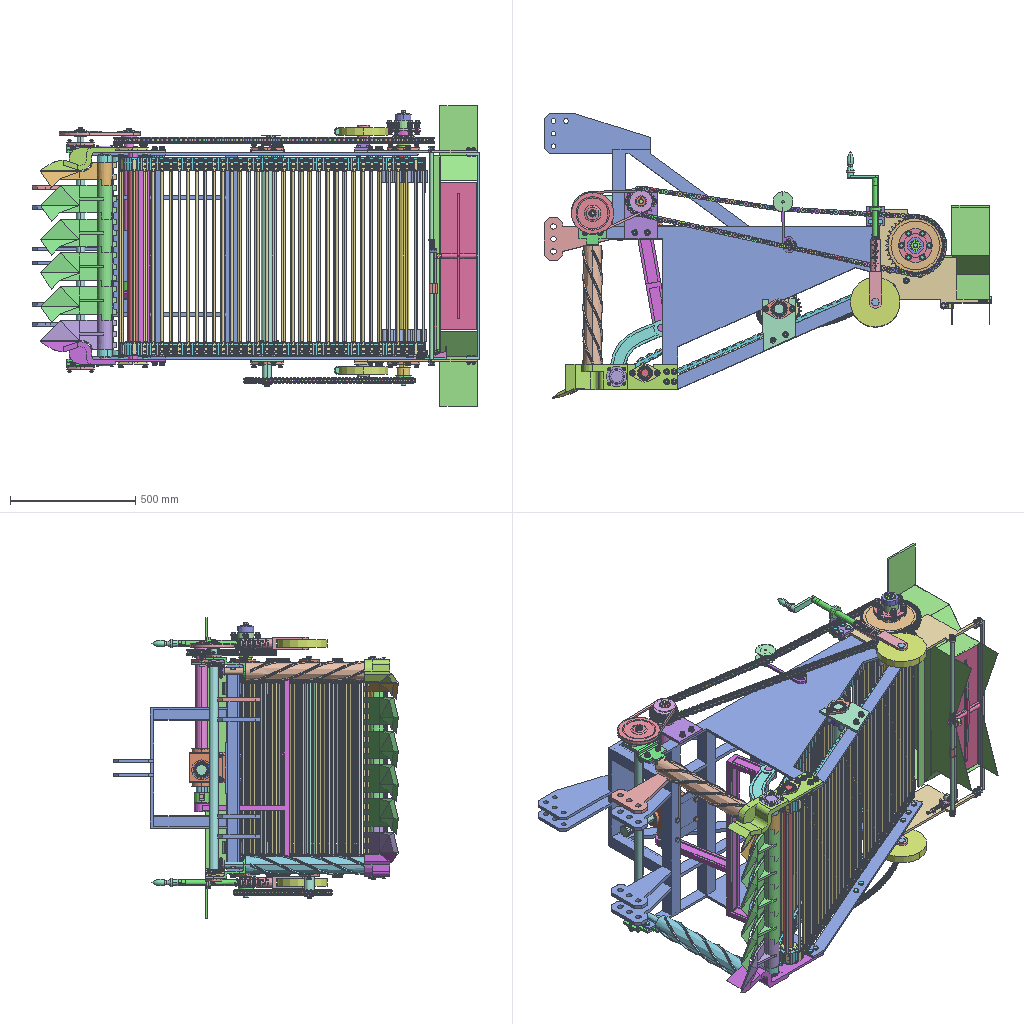Assembly | SolidWorks | 165 different items | 896 placed | box 1790 x 1138 x 1201 mm
Parts list (item | name | quantity | parent item | size | volume | features):
1 | (subassembly) | x1 | in 20 | - | - | -
2 | (subassembly) | x1 | in 20 | - | - | -
3 | (subassembly) | x1 | - | 206.989 x 78.579 x 78.841 mm | 358378 mm3 | -
4 | (subassembly) | x1 | - | - | 9156877 mm3 | features ReferencePattern 399, CompositeCurve 20, LocalLPattern 6
5 | (subassembly) | x1 | - | - | 4579518 mm3 | features ReferencePattern 30, CompositeCurve 4, LocalCirPattern 3, AEMSimFeature 1
6 | (subassembly) | x1 | - | 861 x 69 x 69 mm | 1312162 mm3 | -
7 | (subassembly) | x1 | in 20 | 105 x 134.847 x 502.101 mm | 897409 mm3 | -
8 | (subassembly) | x1 | in 20 | 105 x 134.847 x 502.101 mm | 896444 mm3 | -
9 | (subassembly) | x1 | - | 961.9 x 169.7 x 169.7 mm | 1252859 mm3 | -
10 | (subassembly) | x1 | - | 80.225 x 80.225 x 598.5 mm | 2005498 mm3 | -
11 | (subassembly) | x1 | in 20 | 490.997 x 397.445 x 42.5 mm | 898978 mm3 | -
12 | (subassembly) | x1 | - | 80.225 x 80.225 x 598.5 mm | 2005527 mm3 | -
13 | (subassembly) | x1 | - | - | - | -
14 | (subassembly) | x1 | in 20 | 490.997 x 397.445 x 42.5 mm | 898978 mm3 | -
15 | (subassembly) | x1 | in 20 | 130 x 208 x 42.5 mm | 256605 mm3 | features CompositeCurve 1
16 | (subassembly) | x1 | in 20 | 130 x 208 x 42.5 mm | 256605 mm3 | -
17 | (subassembly) | x1 | - | 950.4 x 178.405 x 179 mm | 1880780 mm3 | features CompositeCurve 6, AEMSimFeature 1
18 | (subassembly) | x1 | - | 859 x 213.314 x 514.351 mm | 4241595 mm3 | features ReferencePattern 3, AEMSimFeature 1, LocalLPattern 1
19 | (subassembly) | x1 | - | 685.4 x 111.714 x 111.249 mm | 1337339 mm3 | features AEMSimFeature 1, CompositeCurve 1
20 | (subassembly) | x1 | - | - | 26128597 mm3 | features CompositeCurve 9, InContextFeatHolder 1
21 | - | x1 | in 20 | 65 x 216.634 x 71 mm | 45722 mm3 | features ICE 2, Extrusion 1
22 | - | x12 | in 5 | 40 x 16 x 16 mm | 3578 mm3 | features BlendCut 1, Cut 1, Fillet 1, LPattern 1, RevCut 1, Revolution 1
23 | - | x1 | in 5 | 1067 x 46 x 46 mm | 1527789 mm3 | features ICE 11, HoleWzd 2, Extrusion 1, MirrorPattern 1
24 | - | x2 | in 5 | 76 x 46 x 46 mm | 30800 mm3 | features Extrusion 1
25 | - | x2 | in 5 | 45 x 5 x 45 mm | 6303 mm3 | features ICE 2, Extrusion 1
26 | - | x2 | in 5 | 20 x 20 x 2 mm | 455.138 mm3 | features Extrusion 1
27 | - | x2 | in 5 | 26.4 x 18.475 x 16 mm | 2773 mm3 | features RevCut 4, Chamfer 1, Extrusion 1, Fillet 1, LPattern 1, Revolution 1
28 | - | x1 | in 5 | 45 x 10 x 8 mm | 3413 mm3 | features Extrusion 1, Fillet 1
29 | - | x1 | in 6 | 861 x 40 x 40 mm | 1030904 mm3 | features ICE 5, Chamfer 1, Extrusion 1
30 | - | x2 | in 6 | 22 x 41 x 41 mm | 7879 mm3 | features Extrusion 1
31 | - | x2 | in 6 | 50 x 69 x 69 mm | 129736 mm3 | features Chamfer 1, Extrusion 1, Fillet 1, ICE 1
32 | - | x1 | in 20 | 15 x 17.5 x 10 mm | 1598 mm3 | features Extrusion 1
33 | - | x2 | in 6 | 40 x 10 x 8 mm | 3014 mm3 | features Extrusion 1, Fillet 1
34 | - | x2 | in 7, 8 | 14 x 62 x 62 mm | 19221 mm3 | features Revolution 5, CirPattern 2, RevCut 2
35 | - | x1 | in 5 | 32 x 239.32 x 240 mm | 513515 mm3 | features CirPattern 2, Cut 2, Revolution 2, Chamfer 1, Fillet 1, MirrorPattern 1
36 | - | x71 | in 4 | 780 x 10 x 15 mm | 63253 mm3 | features ICE 2, Extrusion 1, MirrorSolid 1, RevCut 1, Revolution 1
37 | - | x126 | in 4 | 50 x 5 x 18 mm | 4414 mm3 | features Extrusion 1, HoleWzd 1
38 | - | x2 | in 18 | 300 x 30 x 170 mm | 285435 mm3 | features ICE 4, Extrusion 1
39 | - | x252 | in 4 | 25 x 8.4 x 8.4 mm | 285.936 mm3 | features BlendCut 1, CirPattern 1, LPattern 1, RevCut 1, Revolution 1
40 | - | x2 | in 9 | 22.784 x 63.218 x 63.218 mm | 24670 mm3 | features ICE 2, BlendCut 1, Chamfer 1, CirPattern 1, RefAxis 1, Revolution 1
41 | - | x2 | in 10, 12 | 22.784 x 63.218 x 63.218 mm | 28481 mm3 | features ICE 3, BlendCut 1, Chamfer 1, CirPattern 1, RefAxis 1, Revolution 1
42 | - | x1 | - | 329.455 x 169.695 x 13 mm | 63968 mm3 | features Sweep 1
43 | - | x1 | in 20 | 25 x 28 x 10 mm | 4089 mm3 | features Extrusion 1
44 | - | x1 | in 19 | 23 x 90.5 x 90.5 mm | 81741 mm3 | features Chamfer 1, Cut 1, RevCut 1, Revolution 1
45 | - | x1 | in 7 | 90 x 134.847 x 502.101 mm | 778867 mm3 | features ICE 11, Extrusion 1, HoleWzd 1
46 | - | x1 | in 8 | 90 x 133.847 x 502.101 mm | 777902 mm3 | features ICE 13, Extrusion 1, HoleWzd 1
47 | - | x1 | in 10 | 80.225 x 80.225 x 592.5 mm | 1973629 mm3 | features ICE 4, Extrusion 1, Helix 1, HoleWzd 1, Sweep 1
48 | - | x1 | in 12 | 80.225 x 80.225 x 592.5 mm | 1973636 mm3 | features ICE 4, Extrusion 1, Helix 1, HoleWzd 1, Sweep 1
49 | - | x1 | in 9 | 949 x 35 x 35 mm | 873181 mm3 | features ICE 6, Extrusion 1, HoleWzd 1, MirrorPattern 1
50 | - | x1 | in 9 | 23 x 169.7 x 169.7 mm | 320640 mm3 | features ICE 4, Cut 2, Chamfer 1, Fillet 1, RevCut 1, Revolution 1
51 | - | x1 | in 9 | 18 x 8 x 7 mm | 908.798 mm3 | features Extrusion 1, Fillet 1
52 | - | x2 | in 9 | 36 x 36 x 4.5 mm | 1184 mm3 | features Extrusion 1
53 | - | x2 | in 20 | 110 x 161 x 80 mm | 158190 mm3 | features ICE 4, Fillet 2, Extrusion 1
54 | - | x1 | in 20 | 1540 x 1103 x 825 mm | 15486897 mm3 | features ICE 29, Extrusion 1
55 | - | x1 | in 9 | 30 x 5 x 30 mm | 2498 mm3 | features ICE 2, Extrusion 1
56 | - | x1 | in 9 | 16 x 1.6 x 16 mm | 233.031 mm3 | features Revolution 1
57 | - | x1 | in 9 | 25.3 x 15.011 x 13 mm | 1526 mm3 | features RevCut 4, Chamfer 1, Extrusion 1, Fillet 1, LPattern 1, Revolution 1
58 | - | x2 | in 10, 12 | 19 x 25 x 25 mm | 2965 mm3 | features Cut 1, Fillet 1, LPattern 1, RevCut 1, Revolution 1
59 | - | x2 | in 9 | 14 x 10 x 8 mm | 942.358 mm3 | features Extrusion 1, Fillet 1
60 | - | x2 | in 10, 12 | 14 x 6 x 6 mm | 455.291 mm3 | features Extrusion 1, Fillet 1
61 | - | x2 | in 20 | 200 x 30 x 200 mm | 921272 mm3 | features Revolution 1
62 | - | x1 | in 20 | 70 x 75 x 60 mm | 56680 mm3 | features ICE 2, Extrusion 1
63 | - | x1 | in 20 | 70 x 75 x 100 mm | 66680 mm3 | features ICE 2, Extrusion 1
64 | - | x2 | in 20 | 50 x 275 x 50 mm | 242465 mm3 | features ICE 4, Extrusion 1, Helix 1, SweepCut 1
65 | - | x2 | in 20 | 129 x 33 x 119.886 mm | 71552 mm3 | features Extrusion 1, ICE 1, Revolution 1
66 | - | x2 | in 20 | 50 x 331.25 x 50 mm | 179506 mm3 | features ICE 2, Extrusion 1, Helix 1, HoleWzd 1, Sweep 1
67 | - | x2 | in 20 | 50 x 30 x 30 mm | 35251 mm3 | features Chamfer 1, Extrusion 1
68 | - | x1 | in 5 | 54 x 54 x 31 mm | 40300 mm3 | features ICE 3, CirPattern 1, Extrusion 1, RefAxis 1
69 | - | x1 | in 20 | 180 x 145 x 150 mm | 542429 mm3 | features ICE 8, Extrusion 1
70 | - | x2 | in 20 | 87.5 x 20.785 x 18 mm | 10692 mm3 | features RevCut 4, Chamfer 1, Extrusion 1, Fillet 1, LPattern 1, Revolution 1
71 | - | x2 | in 20 | 37.5 x 20.785 x 18 mm | 5037 mm3 | features RevCut 4, Chamfer 1, Extrusion 1, Fillet 1, LPattern 1, Revolution 1
72 | - | x2 | in 17 | 89.014 x 40 x 79.5 mm | 63655 mm3 | features ICE 2, Chamfer 1, Extrusion 1, HoleWzd 1
73 | - | x6 | in 17 | 41 x 20 x 20 mm | 11584 mm3 | features Extrusion 1, ICE 1
74 | - | x6 | in 17 | 56 x 6 x 6 mm | 1438 mm3 | features LPattern 2, RevCut 2, Chamfer 1, Revolution 1
75 | - | x6 | in 17 | 7.3 x 14.2 x 14.2 mm | 518.031 mm3 | features Cut 2, Boss 1, Chamfer 1, Fillet 1, Revolution 1
76 | - | x1 | in 17 | 935 x 45 x 45 mm | 1400628 mm3 | features ICE 8, Chamfer 1, Extrusion 1, HoleWzd 1
77 | - | x1 | in 18 | 330 x 62.625 x 100 mm | 226101 mm3 | features ICE 17, Extrusion 1, Rib 1
78 | - | x1 | in 5 | 25 x 92.378 x 92.763 mm | 70331 mm3 | features Chamfer 2, Cut 2, Revolution 2, CirPattern 1
79 | - | x1 | in 17 | 20 x 178.394 x 179 mm | 238483 mm3 | features Cut 2, Revolution 2, Chamfer 1, CirPattern 1, Fillet 1, MirrorPattern 1
80 | - | x1 | in 17 | 14 x 10 x 8 mm | 942.358 mm3 | features Extrusion 1, Fillet 1
81 | - | x2 | in 17 | 21 x 46 x 46 mm | 8511 mm3 | features Extrusion 1
82 | - | x2 | in 17 | 32 x 12 x 8 mm | 2813 mm3 | features Extrusion 1, Fillet 1
83 | - | x2 | in 15, 16 | 130 x 208 x 10 mm | 171043 mm3 | features Extrusion 1
84 | - | x1 | in 17 | 45 x 5 x 45 mm | 6303 mm3 | features ICE 2, Extrusion 1
85 | - | x1 | in 17 | 20 x 20 x 2 mm | 455.138 mm3 | features Extrusion 1
86 | - | x1 | in 17 | 26.4 x 18.475 x 16 mm | 2773 mm3 | features RevCut 4, Chamfer 1, Extrusion 1, Fillet 1, LPattern 1, Revolution 1
87 | - | x1 | - | - | 264927 mm3 | features Boss 3, CurvePattern 2, Chamfer 1, CompositeCurve 1, Extrusion 1, MirrorPattern 1, MirrorSolid 1
88 | - | x1 | in 18 | 330 x 62.625 x 140 mm | 410857 mm3 | features ICE 18, Extrusion 1, Rib 1
89 | - | x1 | in 20 | 10.4 x 8 x 8 mm | 174.956 mm3 | features Cut 1, LPattern 1, RevCut 1, Revolution 1
90 | - | x1 | in 18 | 140 x 12 x 8 mm | 13148 mm3 | features Extrusion 1, Fillet 1
91 | - | x1 | in 18 | 110 x 12 x 8 mm | 10277 mm3 | features Extrusion 1, Fillet 1
92 | - | x2 | in 7, 8 | 14 x 62 x 62 mm | 19221 mm3 | features Revolution 5, CirPattern 2, RevCut 2
93 | - | x1 | in 20 | 870 x 42.5 x 203.5 mm | 192112 mm3 | features ICE 2, LPattern 1, MirrorPattern 1, RevCut 1, Sweep 1
94 | - | x1 | in 20 | 19.5 x 19.5 x 35.05 mm | 1610 mm3 | features Helix 3, Cut 2, CompositeCurve 1, Sweep 1
95 | - | x2 | in 20 | 23.219 x 26.75 x 14.8 mm | 3842 mm3 | features Cut 2, Chamfer 1, Extrusion 1
96 | - | x1 | in 20 | 24 x 7 x 7 mm | 343.22 mm3 | features BlendCut 1, Cut 1, Fillet 1, LPattern 1, RevCut 1, Revolution 1
97 | - | x1 | in 19 | 20 x 111.249 x 111.714 mm | 104673 mm3 | features Chamfer 3, Cut 2, Revolution 2, CirPattern 1, ICE 1
98 | - | x2 | in 4 | 1216 x 635.295 x 50 mm | 2018846 mm3 | features ICE 11, Extrusion 1
99 | - | x2 | in 11, 14 | 490.997 x 397.445 x 10 mm | 813417 mm3 | features ICE 5, Cut 1, Extrusion 1
100 | - | x1 | in 20 | 1201 x 475 x 180 mm | 1092637 mm3 | features ICE 9, Extrusion 1
101 | - | x1 | in 20 | 590 x 46 x 155 mm | 188951 mm3 | features ICE 3, Extrusion 1
102 | - | x4 | in 20 | 35.3 x 15.011 x 13 mm | 2140 mm3 | features RevCut 4, Chamfer 1, Extrusion 1, Fillet 1, LPattern 1, Revolution 1
103 | - | x4 | in 20 | 16 x 16 x 1.6 mm | 233.031 mm3 | features Extrusion 1
104 | - | x4 | in 20 | 12.482 x 14.38 x 6.8 mm | 562.42 mm3 | features Cut 2, Chamfer 1, Extrusion 1
105 | - | x1 | in 20 | 825 x 25 x 55 mm | 136025 mm3 | features ICE 2, Extrusion 1, Fillet 1
106 | - | x1 | in 20 | 162.546 x 52 x 20 mm | 43317 mm3 | features ICE 2, Extrusion 1, HoleWzd 1
107 | - | x1 | in 20 | 13 x 13 x 41 mm | 559.424 mm3 | features Helix 3, Cut 2, CompositeCurve 1, Sweep 1
108 | - | x1 | in 20 | 25 x 25 x 25 mm | 9364 mm3 | features Chamfer 1, Extrusion 1, ICE 1
109 | - | x1 | in 19 | 60 x 60 x 75 mm | 108504 mm3 | features ICE 3, Extrusion 1, HoleWzd 1
110 | - | x1 | in 20 | 402 x 65 x 32.5 mm | 47736 mm3 | features ICE 4, Extrusion 1, HoleWzd 1
111 | - | x1 | in 19 | 0.41 x 45 x 45 mm | 234.748 mm3 | features Extrusion 1
112 | - | x1 | in 19 | 119 x 45 x 45 mm | 68134 mm3 | features Extrusion 1
113 | - | x1 | in 19 | 625 x 46 x 46 mm | 866135 mm3 | features ICE 8, HoleWzd 2, Extrusion 1
114 | - | x1 | in 20 | 130 x 190 x 10 mm | 185343 mm3 | features Extrusion 1
115 | - | x1 | in 19 | 45 x 5 x 45 mm | 6303 mm3 | features ICE 2, Extrusion 1
116 | - | x1 | in 19 | 20 x 20 x 2 mm | 455.138 mm3 | features Extrusion 1
117 | - | x2 | in 3, 19 | 26.4 x 18.475 x 16 mm | 2773 mm3 | features RevCut 4, Chamfer 1, Extrusion 1, Fillet 1, LPattern 1, Revolution 1
118 | - | x1 | in 19 | 36 x 10 x 8 mm | 2696 mm3 | features Extrusion 1, Fillet 1
119 | - | x1 | in 19 | 46 x 46 x 12 mm | 4863 mm3 | features Extrusion 1
120 | - | x1 | in 19 | 20 x 12 x 8 mm | 1665 mm3 | features Extrusion 1, Fillet 1
121 | - | x1 | in 18 | 50 x 11 x 50 mm | 7156 mm3 | features Revolution 1
122 | - | x1 | in 19 | 37.5 x 20.785 x 18 mm | 4700 mm3 | features RevCut 4, Chamfer 1, Extrusion 1, Fillet 1, LPattern 1, Revolution 1
123 | - | x1 | - | 794 x 573.5 x 60 mm | 1303043 mm3 | features ICE 14, Extrusion 1
124 | - | x38 | in 20 | 24 x 24 x 2.5 mm | 799.143 mm3 | features Extrusion 1
125 | - | x38 | in 20 | 42.5 x 20.785 x 18 mm | 5603 mm3 | features RevCut 4, Chamfer 1, Extrusion 1, Fillet 1, LPattern 1, Revolution 1
126 | - | x38 | in 20 | 17.386 x 20.03 x 10.8 mm | 1566 mm3 | features Cut 2, Chamfer 1, Extrusion 1
127 | - | x1 | in 5 | 23 x 65 x 65 mm | 53276 mm3 | features ICE 2, Chamfer 1, Cut 1, RevCut 1, Revolution 1
128 | - | x1 | in 5 | 16 x 10 x 8 mm | 1102 mm3 | features Extrusion 1, Fillet 1
129 | - | x8 | in 7, 8 | 22 x 10 x 10 mm | 753.015 mm3 | features BlendCut 1, Cut 1, Fillet 1, LPattern 1, RevCut 1, Revolution 1
130 | - | x1 | in 18 | 859 x 45 x 45 mm | 1051730 mm3 | features ICE 5, Extrusion 1
131 | - | x2 | in 20 | 13 x 55 x 55 mm | 14591 mm3 | features Revolution 5, CirPattern 2, RevCut 2
132 | - | x2 | in 20 | 80 x 5 x 5 mm | 2000 mm3 | features Extrusion 1
133 | - | x7 | in 11, 14, 15, 16, 20 | 15 x 68 x 68 mm | 24020 mm3 | features Revolution 5, CirPattern 2, RevCut 2
134 | - | x2 | in 20 | 110 x 20 x 66 mm | 35046 mm3 | features ICE 3, Extrusion 1
135 | - | x2 | in 7, 8 | 122 x 20 x 72 mm | 37889 mm3 | features ICE 3, Extrusion 1
136 | - | x5 | in 11, 14, 15, 16, 20 | 130 x 20 x 80 mm | 45606 mm3 | features ICE 3, Extrusion 1
137 | - | x4 | in 20 | 41.4 x 18.475 x 16 mm | 3853 mm3 | features RevCut 4, Chamfer 1, Extrusion 1, Fillet 1, LPattern 1, Revolution 1
138 | - | x14 | in 7, 8, 11, 14, 15, 16, 20 | 42.5 x 20.785 x 18 mm | 5603 mm3 | features RevCut 4, Chamfer 1, Extrusion 1, Fillet 1, LPattern 1, Revolution 1
139 | - | x4 | in 20 | 20 x 2 x 20 mm | 455.138 mm3 | features Revolution 1
140 | - | x18 | in 7, 8, 11, 14, 15, 16, 20 | 24 x 2.5 x 24 mm | 799.143 mm3 | features Revolution 1
141 | - | x4 | in 20 | 15.424 x 17.77 x 8.4 mm | 1049 mm3 | features Cut 2, Chamfer 1, Extrusion 1
142 | - | x18 | in 7, 8, 11, 14, 15, 16, 20 | 17.386 x 20.03 x 10.8 mm | 1566 mm3 | features Cut 2, Chamfer 1, Extrusion 1
143 | - | x1 | in 20 | 20 x 30 x 20 mm | 6785 mm3 | features Extrusion 1, ICE 1
144 | - | x2 | in 7, 8 | 82 x 12 x 82 mm | 23262 mm3 | features ICE 2, Revolution 1
145 | - | x1 | in 3 | 196 x 46 x 46 mm | 298815 mm3 | features ICE 4, Extrusion 1, HoleWzd 1
146 | - | x1 | in 3 | 46 x 46 x 7 mm | 2837 mm3 | features Extrusion 1
147 | - | x1 | in 3 | 20 x 12 x 8 mm | 1665 mm3 | features Extrusion 1, Fillet 1
148 | - | x1 | in 3 | 45 x 45 x 3 mm | 4536 mm3 | features Extrusion 1
149 | - | x1 | in 3 | 28.11 x 78.579 x 78.841 mm | 47773 mm3 | features ICE 2, BlendCut 1, Chamfer 1, CirPattern 1, RefAxis 1, Revolution 1
150 | - | x1 | in 19 | 28.614 x 92.976 x 92.976 mm | 84725 mm3 | features ICE 2, BlendCut 1, Chamfer 1, CirPattern 1, RefAxis 1, Revolution 1
151 | - | x1 | in 5 | 95 x 40 x 95 mm | 108607 mm3 | features Extrusion 1, ICE 1
152 | - | x2 | in 5 | 32 x 10 x 8 mm | 2377 mm3 | features Extrusion 1, Fillet 1
153 | - | x6 | in 5 | 24 x 24 x 2.5 mm | 799.143 mm3 | features Extrusion 1
154 | - | x1 | in 20 | 80 x 40 x 80 mm | 76445 mm3 | features Revolution 1
155 | - | x1 | in 5 | 135 x 53 x 135 mm | 118988 mm3 | features ICE 3, Extrusion 1, HoleWzd 1
156 | - | x1 | in 5 | 135 x 3 x 135 mm | 31516 mm3 | features Extrusion 1, HoleWzd 1
157 | - | x1 | in 5 | 56 x 20 x 56 mm | 16886 mm3 | features Extrusion 1, ICE 1
158 | - | x6 | in 5 | 21 x 21 x 20 mm | 1917 mm3 | features Helix 3, Cut 2, CompositeCurve 1, Sweep 1
159 | - | x6 | in 5 | 24.7 x 24.7 x 56.9 mm | 6988 mm3 | features Cut 2, Boss 1, Extrusion 1, LPattern 1, RevCut 1, Revolution 1
160 | - | x6 | in 5 | 17.386 x 20.03 x 10.8 mm | 1566 mm3 | features Cut 2, Chamfer 1, Extrusion 1
161 | - | x1 | - | - | 653125 mm3 | features Boss 3, CurvePattern 2, Chamfer 1, CompositeCurve 1, Extrusion 1, MirrorPattern 1, MirrorSolid 1
162 | - | x2 | in 5 | 188.466 x 50 x 187.3 mm | 763094 mm3 | features ICE 2, CirPattern 1, Extrusion 1
163 | - | x2 | in 5 | 32 x 12 x 8 mm | 2813 mm3 | features Extrusion 1, Fillet 1
164 | - | x4 | in 5 | 19 x 120 x 120 mm | 91296 mm3 | features Chamfer 1, Extrusion 1, HoleWzd 1, ICE 1
165 | - | x4 | in 18 | 330 x 62.625 x 170 mm | 487864 mm3 | features ICE 14, Extrusion 1, Rib 1
Mates (type | each side: item.copy, entity, surface, feature), first 531 of 899 lines:
In the top assembly
Concentric | 133.1 face cylinder Boss-Revolve 4 | 113.1 face cylinder Boss-Extrude 2
Coincident | 133.1 face plane Boss-Revolve 4 | 119.1 edge
Concentric | 131.1 face cylinder Boss-Revolve 4 | 49.1 face cylinder Mirror 1
Coincident | 131.2 face plane Boss-Revolve 4 | 52.1 face plane Boss-Extrude 1
Concentric | 46.1 face cylinder Cut-Extrude 17 | 47.1 face cylinder Boss-Extrude 1
Coincident | 46.1 face plane Cut-Extrude 17 | 47.1 face plane Boss-Extrude 1
Concentric | 53.1 face cylinder Cut-Extrude 1 | 48.1 face cylinder Boss-Extrude 3
Coincident | 45.1 face plane Cut-Extrude 5 | 48.1 face plane Boss-Extrude 1
Concentric | 133.2 face cylinder Boss-Revolve 4 | 23.1 face cylinder Boss-Extrude 7
Coincident | 133.2 face plane Boss-Revolve 4 | 24.1 face plane Boss-Extrude 1
GearDim | assembly edge | 35.1 edge
Concentric | 92.1 face cylinder Boss-Revolve 4 | 29.1 face cylinder Boss-Extrude 5
Coincident | 92.1 face plane Boss-Revolve 4 | 30.1 face plane Boss-Extrude 1
Concentric | assembly face | assembly face
Coincident | assembly face | assembly face
Concentric | 133.3 face cylinder Boss-Revolve 4 | 76.1 face cylinder Boss-Extrude 7
Coincident | 133.3 face plane Boss-Revolve 4 | 81.1 face plane Boss-Extrude 1
Concentric | 92.2 face cylinder Boss-Revolve 4 | 130.1 face cylinder Boss-Extrude 5
Coincident | 92.2 face plane Boss-Revolve 4 | 130.1 face plane Boss-Extrude 4
Concentric | 109.1 face cylinder Boss-Extrude 3 | 123.1 face cylinder Boss-Extrude 1
Coincident | 109.1 face plane Boss-Extrude 2 | 123.1 face plane Boss-Extrude 1
Concentric | 38.1 face cylinder Boss-Extrude 2 | 123.1 face cylinder Boss-Extrude 7
Concentric | 133.4 face cylinder Boss-Revolve 4 | 145.1 face cylinder Boss-Extrude 2
Coincident | 133.4 face plane Boss-Revolve 4 | 145.1 face plane Boss-Extrude 3
GearDim | 149.1 edge | 150.1 edge
Coincident | 31.1 face plane Boss-Extrude 1 | 98.1 face plane Boss-Extrude 2
Concentric | 31.1 face cylinder Boss-Extrude 2 | 98.1 face cylinder Boss-Extrude 2
DistanceDim | 24.1 face cylinder Boss-Extrude 1 | 98.2 face cylinder Boss-Extrude 2
Coincident | 97.1 face plane Revolve 1 | 161.1 face plane 曲线Pattern 1
Coincident | 44.1 face cone Cut-Revolve 1 | 42.1 edge
Parallel | 99.1 face plane Boss-Extrude 1 | 128.1 face plane Base-Extrude
Concentric | 87.1 edge | assembly select_type:10
Parallel | 46.1 face plane Boss-Extrude 1 | 33.1 face plane Base-Extrude
Parallel | 53.2 face plane Boss-Extrude 1 | 60.1 face plane Base-Extrude
Parallel | 59.1 face plane Base-Extrude | 114.1 face plane Boss-Extrude 1
Parallel | 53.1 face plane Boss-Extrude 1 | 60.2 face plane Base-Extrude
Coincident | 78.1 face plane Revolve 1 | 87.1 face plane 曲线Pattern 1
In subassembly 18
Coincident | 130.2 face plane Boss-Extrude 3 | 38.2 face plane Boss-Extrude 1
Coincident | 130.2 axis | 88.1 axis
Coincident | 38.2 face plane Boss-Extrude 1 | 88.1 face plane Boss-Extrude 24
Coincident | 130.2 axis | 165.1 axis
Coincident | 88.1 face plane Cut-Extrude 1 | 165.1 face plane Cut-Extrude 2
Coincident | 88.1 face plane Boss-Extrude 1 | 165.1 face plane Boss-Extrude 2
Coincident | 130.2 axis | 77.1 axis
Coincident | 77.1 face plane Cut-Extrude 2 | 165.2 face plane Cut-Extrude 1
Coincident | 77.1 face plane Boss-Extrude 2 | 165.2 face plane Boss-Extrude 1
Coincident | 130.2 axis | 38.3 axis
Parallel | 130.2 face plane Cut-Extrude 1 | 38.3 face plane Boss-Extrude 1
Coincident | 77.1 face plane Boss-Extrude 24 | 38.3 face plane Boss-Extrude 1
Coincident | 130.2 axis | 121.1 axis
Coincident | 38.3 face plane Boss-Extrude 1 | 121.1 face plane Revolve 1
Coincident | 130.2 face plane Cut-Extrude 1 | 91.1 face plane Base-Extrude | 2 times
Concentric | 130.2 face cylinder Cut-Extrude 1 | 91.1 face cylinder Base-Extrude
Coincident | 130.2 face plane Cut-Extrude 1 | 90.1 face plane Base-Extrude | 2 times
Concentric | 130.2 face cylinder Cut-Extrude 1 | 90.1 face cylinder Base-Extrude
Coincident | 88.1 face plane Cut-Extrude 16 | 90.1 face plane Base-Extrude
Coincident | 38.2 face plane Boss-Extrude 1 | 90.1 face plane Base-Extrude
Concentric | 130.2 face cylinder Boss-Extrude 1 | 38.2 face cylinder Boss-Extrude 1
In subassembly 3
Concentric | 145.2 face cylinder Boss-Extrude 1 | 149.2 face cylinder Cut-Extrude 1
Coincident | 145.2 face plane Cut-Extrude 1 | 147.1 face plane Base-Extrude | 2 times
Concentric | 145.2 face cylinder Cut-Extrude 1 | 147.1 face cylinder Base-Extrude
Concentric | 145.2 face cylinder Boss-Extrude 2 | 146.1 face cylinder Boss-Extrude 1
DistanceDim | 145.2 face plane Boss-Extrude 3 | 146.1 face plane Boss-Extrude 1
Parallel | 149.2 face plane Cut-Extrude 1 | 147.1 face plane Base-Extrude
Coincident | 149.2 face plane Boss-Extrude 1 | 146.1 face plane Boss-Extrude 1
Coincident | 149.2 face plane Revolve 1 | 148.1 face plane Boss-Extrude 1
Concentric | 145.2 face cylinder M10 Tapped Hole 1 | 148.1 face cylinder Boss-Extrude 1
Concentric | 148.1 face cylinder Boss-Extrude 1 | 117.1 face cylinder Boss-Revolve 1
Coincident | 148.1 face plane Boss-Extrude 1 | 117.1 face plane Base-Extrude
In subassembly 9
Coincident | 49.2 face plane Cut-Extrude 1 | 59.2 face plane Base-Extrude | 2 times
Concentric | 49.2 face cylinder Cut-Extrude 1 | 59.2 face cylinder Base-Extrude
Coincident | 49.2 face plane Cut-Extrude 1 | 59.3 face plane Base-Extrude | 2 times
Concentric | 49.2 face cylinder Cut-Extrude 1 | 59.3 face cylinder Base-Extrude
Coincident | 49.2 face plane Cut-Extrude 2 | 51.1 face plane Base-Extrude | 2 times
Concentric | 49.2 face cylinder Cut-Extrude 2 | 51.1 face cylinder Base-Extrude
Concentric | 49.2 face cylinder Boss-Extrude 5 | 50.1 face cylinder Revolve 1
Coincident | 51.1 face plane Base-Extrude | 50.1 face plane Cut-Extrude 1
Coincident | 49.2 face plane Boss-Extrude 4 | 50.1 face plane Revolve 1
Coincident | 50.1 face plane Revolve 1 | 55.1 face plane Boss-Extrude 1
Concentric | 49.2 face cylinder M8 Tapped Hole 1 | 55.1 face cylinder Cut-Extrude 1
Coincident | 55.1 face plane Boss-Extrude 2 | 56.1 face plane Base-Revolve
Concentric | 49.2 face cylinder M8 Tapped Hole 1 | 56.1 face cylinder Base-Revolve
Coincident | 57.1 face plane Base-Extrude | 56.1 face plane Base-Revolve
Concentric | 49.2 face cylinder M8 Tapped Hole 1 | 57.1 face cylinder Cut-Revolve 3
Concentric | 49.2 face cylinder Boss-Extrude 3 | 52.2 face cylinder Boss-Extrude 1
Concentric | 49.2 face cylinder Mirror 1 | 52.3 face cylinder Boss-Extrude 1
In subassembly 6
Coincident | 29.2 face plane Cut-Extrude 1 | 33.2 face plane Base-Extrude | 2 times
Concentric | 29.2 face cylinder Cut-Extrude 1 | 33.2 face cylinder Base-Extrude
Coincident | 29.2 face plane Cut-Extrude 1 | 33.3 face plane Base-Extrude | 2 times
Concentric | 29.2 face cylinder Cut-Extrude 1 | 33.3 face cylinder Base-Extrude
Coincident | 29.2 axis | 31.2 axis
Coincident | 33.3 face plane Base-Extrude | 31.2 face plane Boss-Extrude 1
Coincident | 29.2 face plane Boss-Extrude 1 | 31.2 face plane Boss-Extrude 1
Coincident | 29.2 axis | 31.3 axis
Coincident | 33.2 face plane Base-Extrude | 31.3 face plane Boss-Extrude 1
Coincident | 29.2 face plane Boss-Extrude 1 | 31.3 face plane Boss-Extrude 1
Coincident | 29.2 axis | 30.2 axis
Coincident | 31.3 face plane Boss-Extrude 1 | 30.2 face plane Boss-Extrude 1
Coincident | 29.2 axis | 30.3 axis
Coincident | 31.2 face plane Boss-Extrude 1 | 30.3 face plane Boss-Extrude 1
In subassembly 20
Coincident | 46.2 face plane Boss-Extrude 1 | 54.1 face plane Boss-Extrude 2
Coincident | 54.1 axis | 46.2 axis | 2 times
Coincident | 45.2 face plane Boss-Extrude 1 | 54.1 face plane Boss-Extrude 4
Coincident | 54.1 axis | 45.2 axis | 2 times
Coincident | 54.1 axis | 20.1 axis | 4 times
Coincident | 20.1 face | 54.1 face plane Boss-Extrude 4
Coincident | 54.1 face plane Boss-Extrude 4 | 83.1 face plane Boss-Extrude 1
Coincident | 54.1 axis | 83.1 axis
DistanceDim | 83.1 axis | 54.1 axis
Coincident | 54.1 face plane Boss-Extrude 2 | 83.2 face plane Boss-Extrude 1
Coincident | 54.1 axis | 83.2 axis
DistanceDim | 54.1 axis | 83.2 axis
Coincident | 45.2 face plane Boss-Extrude 8 | 124.1 face plane Extrude 1
Coincident | 45.2 axis | 124.1 axis
Coincident | 45.2 face plane Boss-Extrude 8 | 124.2 face plane Extrude 1
Coincident | 45.2 axis | 124.2 axis
Coincident | 45.2 face plane Boss-Extrude 8 | 124.3 face plane Extrude 1
Coincident | 45.2 axis | 124.3 axis
Coincident | 45.2 face plane Boss-Extrude 8 | 124.4 face plane Extrude 1
Coincident | 54.1 axis | 124.4 axis
Coincident | 124.1 face plane Extrude 1 | 126.1 face plane Base-Extrude
Coincident | 54.1 axis | 126.1 axis
Coincident | 124.2 face plane Extrude 1 | 126.2 face plane Base-Extrude
Coincident | 54.1 axis | 126.2 axis
Coincident | 124.4 face plane Extrude 1 | 126.3 face plane Base-Extrude
Coincident | 54.1 axis | 126.3 axis
Coincident | 124.4 face plane Extrude 1 | 126.4 face plane Base-Extrude
Coincident | 54.1 axis | 126.4 axis
Coincident | 54.1 face plane Boss-Extrude 4 | 125.1 face plane Base-Extrude
Coincident | 54.1 axis | 125.1 axis
Coincident | 54.1 face plane Boss-Extrude 4 | 125.2 face plane Base-Extrude
Coincident | 54.1 axis | 125.2 axis
Coincident | 54.1 face plane Boss-Extrude 4 | 125.3 face plane Base-Extrude
Coincident | 54.1 axis | 125.3 axis
Coincident | 54.1 face plane Boss-Extrude 4 | 125.4 face plane Base-Extrude
Coincident | 54.1 axis | 125.4 axis
Coincident | 54.1 axis | 124.5 axis
Coincident | 54.1 axis | 124.6 axis
Coincident | 124.5 axis | 126.5 axis
Coincident | 124.6 axis | 126.6 axis
Coincident | 124.6 face plane Extrude 1 | 126.6 face plane Base-Extrude
Coincident | 124.5 face plane Extrude 1 | 126.5 face plane Base-Extrude
Coincident | 126.6 axis | 125.5 axis
Coincident | 126.5 axis | 125.6 axis
Coincident | 54.1 face plane Boss-Extrude 2 | 125.7 face plane Base-Extrude
Coincident | 54.1 face plane Boss-Extrude 2 | 125.8 face plane Base-Extrude
Coincident | 54.1 face plane Boss-Extrude 2 | 125.9 face plane Base-Extrude
Coincident | 54.1 face plane Boss-Extrude 2 | 125.10 face plane Base-Extrude
Coincident | 54.1 axis | 125.10 axis
Coincident | 54.1 axis | 125.9 axis
Coincident | 54.1 axis | 125.8 axis
Coincident | 54.1 axis | 125.7 axis
Coincident | 46.2 face plane Boss-Extrude 11 | 124.7 face plane Extrude 1
Coincident | 54.1 axis | 124.7 axis
Coincident | 46.2 face plane Boss-Extrude 11 | 124.8 face plane Extrude 1
Coincident | 54.1 axis | 124.8 axis
Coincident | 46.2 face plane Boss-Extrude 11 | 124.9 face plane Extrude 1
Coincident | 46.2 axis | 124.9 axis
Coincident | 46.2 face plane Boss-Extrude 11 | 124.10 face plane Extrude 1
Coincident | 46.2 axis | 124.10 axis
Coincident | 124.9 face plane Extrude 1 | 126.7 face plane Base-Extrude
Coincident | 46.2 axis | 126.7 axis
Coincident | 124.10 face plane Extrude 1 | 126.8 face plane Base-Extrude
Coincident | 46.2 axis | 126.8 axis
Coincident | 124.7 face plane Extrude 1 | 126.9 face plane Base-Extrude
Coincident | 46.2 axis | 126.9 axis
Coincident | 124.8 face plane Extrude 1 | 126.10 face plane Base-Extrude
Coincident | 46.2 axis | 126.10 axis
Coincident | 54.1 axis | 124.11 axis
Coincident | 54.1 axis | 124.12 axis
Coincident | 124.11 face plane Extrude 1 | 126.11 face plane Base-Extrude
Coincident | 124.12 face plane Extrude 1 | 126.12 face plane Base-Extrude
Coincident | 54.1 axis | 126.11 axis
Coincident | 54.1 axis | 126.12 axis
Coincident | 126.12 axis | 125.11 axis
Coincident | 126.11 axis | 125.12 axis
Coincident | 54.1 face plane Boss-Extrude 2 | 20.1 face
Coincident | 54.1 face plane Boss-Extrude 4 | 125.5 face plane Base-Extrude
Coincident | 54.1 face plane Boss-Extrude 4 | 125.6 face plane Base-Extrude
Coincident | 83.1 face plane Boss-Extrude 1 | 124.6 face plane Extrude 1
Coincident | 83.1 face plane Boss-Extrude 1 | 124.5 face plane Extrude 1
Coincident | 83.2 face plane Boss-Extrude 1 | 124.12 face plane Extrude 1
Coincident | 83.2 face plane Boss-Extrude 1 | 124.11 face plane Extrude 1
Coincident | 54.1 face plane Boss-Extrude 2 | 125.12 face plane Base-Extrude
Coincident | 54.1 face plane Boss-Extrude 2 | 125.11 face plane Base-Extrude
Concentric | 54.1 face cylinder Boss-Extrude 4 | 99.2 face cylinder Boss-Extrude 1
Coincident | 54.1 face plane Boss-Extrude 4 | 99.2 face plane Boss-Extrude 1
Concentric | 54.1 face cylinder Boss-Extrude 4 | 99.2 face cylinder Cut-Extrude 1
Concentric | 54.1 face cylinder Boss-Extrude 2 | 99.3 face cylinder Boss-Extrude 1
Concentric | 54.1 face cylinder Boss-Extrude 2 | 99.3 face cylinder Cut-Extrude 1
Coincident | 54.1 face plane Boss-Extrude 2 | 99.3 face plane Boss-Extrude 1
Coincident | 99.3 axis | 124.13 axis
Coincident | 54.1 axis | 124.14 axis
Coincident | 99.3 axis | 124.15 axis
Coincident | 99.3 axis | 124.16 axis
Coincident | 99.3 axis | 124.17 axis
Coincident | 54.1 axis | 126.13 axis
Coincident | 99.3 axis | 126.14 axis
Coincident | 99.3 axis | 126.15 axis
Coincident | 54.1 axis | 126.16 axis
Coincident | 54.1 axis | 126.17 axis
Coincident | 99.3 face plane Boss-Extrude 1 | 124.17 face plane Extrude 1
Coincident | 99.3 face plane Boss-Extrude 1 | 124.16 face plane Extrude 1
Coincident | 99.3 face plane Boss-Extrude 1 | 124.15 face plane Extrude 1
Coincident | 99.3 face plane Boss-Extrude 1 | 124.14 face plane Extrude 1
Coincident | 99.3 face plane Boss-Extrude 1 | 124.13 face plane Extrude 1
Coincident | 124.13 face plane Extrude 1 | 126.17 face plane Base-Extrude
Coincident | 124.14 face plane Extrude 1 | 126.16 face plane Base-Extrude
Coincident | 124.15 face plane Extrude 1 | 126.15 face plane Base-Extrude
Coincident | 124.16 face plane Extrude 1 | 126.14 face plane Base-Extrude
Coincident | 124.17 face plane Extrude 1 | 126.13 face plane Base-Extrude
Coincident | 54.1 axis | 125.13 axis
Coincident | 54.1 axis | 125.14 axis
Coincident | 54.1 axis | 125.15 axis
Coincident | 54.1 axis | 125.16 axis
Coincident | 54.1 axis | 125.17 axis
Coincident | 54.1 face plane Boss-Extrude 2 | 125.15 face plane Base-Extrude
Coincident | 54.1 face plane Boss-Extrude 2 | 125.13 face plane Base-Extrude
Coincident | 54.1 face plane Boss-Extrude 2 | 125.14 face plane Base-Extrude
Coincident | 54.1 face plane Boss-Extrude 2 | 125.17 face plane Base-Extrude
Coincident | 54.1 face plane Boss-Extrude 2 | 125.16 face plane Base-Extrude
Coincident | 54.1 axis | 125.18 axis
Coincident | 54.1 axis | 125.19 axis
Coincident | 54.1 axis | 125.20 axis
Coincident | 54.1 axis | 125.21 axis
Coincident | 54.1 axis | 125.22 axis
Coincident | 99.2 axis | 124.18 axis
Coincident | 54.1 axis | 124.19 axis
Coincident | 54.1 axis | 124.20 axis
Coincident | 54.1 axis | 124.21 axis
Coincident | 54.1 axis | 124.22 axis
Coincident | 54.1 axis | 126.18 axis
Coincident | 54.1 axis | 126.19 axis
Coincident | 99.2 axis | 126.20 axis
Coincident | 99.2 axis | 126.21 axis
Coincident | 54.1 axis | 126.22 axis
Coincident | 54.1 face plane Boss-Extrude 4 | 125.22 face plane Base-Extrude
Coincident | 54.1 face plane Boss-Extrude 4 | 125.21 face plane Base-Extrude
Coincident | 54.1 face plane Boss-Extrude 4 | 125.20 face plane Base-Extrude
Coincident | 54.1 face plane Boss-Extrude 4 | 125.19 face plane Base-Extrude
Coincident | 54.1 face plane Boss-Extrude 4 | 125.18 face plane Base-Extrude
Coincident | 99.2 face plane Boss-Extrude 1 | 124.20 face plane Extrude 1
Coincident | 99.2 face plane Boss-Extrude 1 | 124.19 face plane Extrude 1
Coincident | 99.2 face plane Boss-Extrude 1 | 124.18 face plane Extrude 1
Coincident | 99.2 face plane Boss-Extrude 1 | 124.22 face plane Extrude 1
Coincident | 99.2 face plane Boss-Extrude 1 | 124.21 face plane Extrude 1
Coincident | 124.21 face plane Extrude 1 | 126.18 face plane Base-Extrude
Coincident | 124.22 face plane Extrude 1 | 126.19 face plane Base-Extrude
Coincident | 124.20 face plane Extrude 1 | 126.20 face plane Base-Extrude
Coincident | 124.19 face plane Extrude 1 | 126.21 face plane Base-Extrude
Coincident | 124.18 face plane Extrude 1 | 126.22 face plane Base-Extrude
Concentric | 54.1 face cylinder Boss-Extrude 2 | 114.2 face cylinder Boss-Extrude 1 | 2 times
Coincident | 54.1 face plane Boss-Extrude 2 | 114.2 face plane Boss-Extrude 1
Concentric | 114.2 face cylinder Boss-Extrude 1 | 136.1 face cylinder Boss-Extrude 1 | 2 times
Coincident | 114.2 face plane Boss-Extrude 1 | 136.1 face plane Boss-Extrude 1
Concentric | 133.5 face cylinder Boss-Revolve 3 | 136.1 face cylinder Cut-Extrude 1
Coincident | 133.5 face plane Boss-Revolve 3 | 136.1 face plane Cut-Extrude 1
Coincident | 53.3 face plane Boss-Extrude 1 | 54.1 face plane Boss-Extrude 2
Concentric | 54.1 face cylinder Boss-Extrude 2 | 53.3 face cylinder Boss-Extrude 1 | 2 times
Concentric | 54.1 face cylinder Boss-Extrude 4 | 53.4 face cylinder Boss-Extrude 1 | 2 times
Coincident | 54.1 face plane Boss-Extrude 4 | 53.4 face plane Boss-Extrude 1
Concentric | 53.3 face cylinder Boss-Extrude 4 | 134.1 face cylinder Boss-Extrude 1 | 3 times
Coincident | 53.3 face plane Boss-Extrude 4 | 134.1 face plane Boss-Extrude 1
Concentric | 134.1 face cylinder Cut-Extrude 1 | 131.3 face cylinder Boss-Revolve 3
Coincident | 134.1 face plane Cut-Extrude 1 | 131.3 face plane Boss-Revolve 3
Concentric | 53.4 face cylinder Boss-Extrude 4 | 134.2 face cylinder Boss-Extrude 1 | 3 times
Coincident | 53.4 face plane Boss-Extrude 4 | 134.2 face plane Boss-Extrude 1
Concentric | 134.2 face cylinder Cut-Extrude 1 | 131.4 face cylinder Boss-Revolve 3
Coincident | 134.2 face plane Cut-Extrude 1 | 131.4 face plane Boss-Revolve 3
Coincident | 114.2 face plane Boss-Extrude 1 | 124.23 face plane Extrude 1
Coincident | 114.2 face plane Boss-Extrude 1 | 124.24 face plane Extrude 1
Concentric | 114.2 face cylinder Boss-Extrude 1 | 124.24 face cylinder Extrude 1
Concentric | 114.2 face cylinder Boss-Extrude 1 | 124.23 face cylinder Extrude 1
Coincident | 53.3 face plane Boss-Extrude 1 | 124.25 face plane Extrude 1
Coincident | 53.3 face plane Boss-Extrude 1 | 124.26 face plane Extrude 1
Concentric | 53.3 face cylinder Boss-Extrude 1 | 124.26 face cylinder Extrude 1
Concentric | 53.3 face cylinder Boss-Extrude 1 | 124.25 face cylinder Extrude 1
Coincident | 124.24 face plane Extrude 1 | 126.23 face plane Base-Extrude
Concentric | 114.2 face cylinder Boss-Extrude 1 | 126.23 face cone Chamfer 1
Coincident | 124.23 face plane Extrude 1 | 126.24 face plane Base-Extrude
Concentric | 114.2 face cylinder Boss-Extrude 1 | 126.24 face cone Chamfer 1
Coincident | 124.25 face plane Extrude 1 | 126.25 face plane Base-Extrude
Coincident | 53.3 face cylinder Boss-Extrude 1 | 126.25 edge
Coincident | 124.26 face plane Extrude 1 | 126.26 face plane Base-Extrude
Concentric | 53.3 face cylinder Boss-Extrude 1 | 126.26 edge
Coincident | 54.1 axis | 125.23 axis
Coincident | 54.1 axis | 125.24 axis
Coincident | 54.1 axis | 125.25 axis
Coincident | 54.1 axis | 125.26 axis
Coincident | 54.1 face plane Boss-Extrude 2 | 125.26 face plane Base-Extrude
Coincident | 54.1 face plane Boss-Extrude 2 | 125.25 face plane Base-Extrude
Coincident | 54.1 face plane Boss-Extrude 2 | 125.23 face plane Base-Extrude
Coincident | 54.1 face plane Boss-Extrude 2 | 125.24 face plane Base-Extrude
Concentric | 139.1 face cylinder Base-Revolve | 134.1 face cylinder Boss-Extrude 1
Concentric | 134.1 face cylinder Boss-Extrude 1 | 139.2 face cylinder Base-Revolve
Coincident | 134.1 face plane Boss-Extrude 1 | 139.2 face plane Base-Revolve
Coincident | 134.1 face plane Boss-Extrude 1 | 139.1 face plane Base-Revolve
Coincident | 141.1 face plane Base-Extrude | 139.1 face plane Base-Revolve
Coincident | 141.2 face plane Base-Extrude | 139.2 face plane Base-Revolve
Concentric | 141.2 edge | 139.2 face cylinder Base-Revolve
Concentric | 134.1 face cylinder Boss-Extrude 1 | 141.1 edge
Concentric | 53.3 face cylinder Boss-Extrude 4 | 137.1 face cylinder Boss-Revolve 1
Concentric | 53.3 face cylinder Boss-Extrude 4 | 137.2 face cylinder Boss-Revolve 1
Coincident | 53.3 face plane Boss-Extrude 4 | 137.1 face plane Base-Extrude
Coincident | 53.3 face plane Boss-Extrude 4 | 137.2 face plane Base-Extrude
Coincident | 53.4 face plane Boss-Extrude 1 | 124.27 face plane Extrude 1
Coincident | 53.4 face plane Boss-Extrude 1 | 124.28 face plane Extrude 1
Coincident | 124.28 face plane Extrude 1 | 126.27 face plane Base-Extrude
Coincident | 124.27 face plane Extrude 1 | 126.28 face plane Base-Extrude
Concentric | 53.4 face cylinder Boss-Extrude 1 | 124.27 face cylinder Extrude 1
Concentric | 53.4 face cylinder Boss-Extrude 1 | 124.28 face cylinder Extrude 1
Concentric | 53.4 face cylinder Boss-Extrude 1 | 126.28 face cone Chamfer 1
Concentric | 53.4 face cylinder Boss-Extrude 1 | 126.27 edge
Coincident | 54.1 face plane Boss-Extrude 4 | 125.27 face plane Base-Extrude
Coincident | 54.1 face plane Boss-Extrude 4 | 125.28 face plane Base-Extrude
Concentric | 54.1 face cylinder Boss-Extrude 4 | 125.27 face cylinder Boss-Revolve 1
Concentric | 54.1 face cylinder Boss-Extrude 4 | 125.28 face cylinder Boss-Revolve 1
Coincident | 134.2 face plane Boss-Extrude 1 | 139.3 face plane Base-Revolve
Coincident | 134.2 face plane Boss-Extrude 1 | 139.4 face plane Base-Revolve
Concentric | 134.2 face cylinder Boss-Extrude 1 | 139.4 face cylinder Base-Revolve
Concentric | 134.2 face cylinder Boss-Extrude 1 | 139.3 face cylinder Base-Revolve
Concentric | 141.3 face cylinder Base-Extrude | 139.4 face cylinder Base-Revolve
Concentric | 134.2 face cylinder Boss-Extrude 1 | 141.4 face cylinder Base-Extrude
Concentric | 134.2 face cylinder Boss-Extrude 1 | 137.3 face cylinder Boss-Revolve 1
Concentric | 134.2 face cylinder Boss-Extrude 1 | 137.4 face cylinder Boss-Revolve 1
Coincident | 141.3 face plane Base-Extrude | 139.4 face plane Base-Revolve
Coincident | 141.4 face plane Base-Extrude | 139.3 face plane Base-Revolve
Coincident | 53.4 face plane Boss-Extrude 4 | 137.3 face plane Base-Extrude
Coincident | 53.4 face plane Boss-Extrude 4 | 137.4 face plane Base-Extrude
Concentric | 136.1 face cylinder Boss-Extrude 1 | 140.1 face cylinder Base-Revolve
Concentric | 136.1 face cylinder Boss-Extrude 1 | 140.2 face cylinder Base-Revolve
Concentric | 136.1 face cylinder Boss-Extrude 1 | 142.1 face cylinder Base-Extrude
Concentric | 136.1 face cylinder Boss-Extrude 1 | 142.2 face cylinder Base-Extrude
Concentric | 136.1 face cylinder Boss-Extrude 1 | 138.1 face cylinder Boss-Revolve 1
Concentric | 136.1 face cylinder Boss-Extrude 1 | 138.2 face cylinder Boss-Revolve 1
Coincident | 136.1 face plane Boss-Extrude 1 | 140.1 face plane Base-Revolve
Coincident | 136.1 face plane Boss-Extrude 1 | 140.2 face plane Base-Revolve
Coincident | 142.1 face plane Base-Extrude | 140.2 face plane Base-Revolve
Coincident | 142.2 face plane Base-Extrude | 140.1 face plane Base-Revolve
Coincident | 114.2 face plane Boss-Extrude 1 | 138.2 face plane Base-Extrude
Coincident | 114.2 face plane Boss-Extrude 1 | 138.1 face plane Base-Extrude
Coincident | 54.1 face plane Boss-Extrude 15 | 71.1 face plane Base-Extrude
Coincident | 54.1 face plane Boss-Extrude 15 | 71.2 face plane Base-Extrude
Concentric | 54.1 face cylinder Boss-Extrude 15 | 71.1 face cylinder Cut-Revolve 3
Concentric | 54.1 face cylinder Boss-Extrude 15 | 71.2 face cylinder Cut-Revolve 3
Concentric | 142.3 face cylinder Base-Extrude | 140.3 face cylinder Base-Revolve
Coincident | 142.3 face plane Base-Extrude | 140.3 face plane Base-Revolve
Coincident | 142.4 face plane Base-Extrude | 140.4 face plane Base-Revolve
Concentric | 142.4 face cylinder Base-Extrude | 140.4 face cylinder Base-Revolve
Coincident | 142.5 face plane Base-Extrude | 140.5 face plane Base-Revolve
Coincident | 142.6 face plane Base-Extrude | 140.6 face plane Base-Revolve
Coincident | 54.1 face plane Boss-Extrude 1 | 70.1 face plane Base-Extrude
Coincident | 54.1 face plane Boss-Extrude 1 | 70.2 face plane Base-Extrude
Concentric | 142.5 face cylinder Base-Extrude | 70.2 face cylinder Boss-Revolve 1
Concentric | 142.6 face cylinder Base-Extrude | 70.1 face cylinder Boss-Revolve 1
Coincident | 99.3 face plane Boss-Extrude 1 | 105.1 face plane Boss-Extrude 1
Concentric | 99.3 face cylinder Boss-Extrude 2 | 105.1 face cylinder Boss-Extrude 3 | 2 times
Tangent | 101.1 face cylinder Boss-Extrude 1 | 105.1 face cylinder Boss-Extrude 1
Concentric | 100.1 face cylinder Cut-Extrude 1 | 105.1 face cylinder Boss-Extrude 1
Coincident | 100.1 face plane Boss-Extrude 2 | 105.1 face plane Boss-Extrude 1
Coincident | 101.1 face plane Boss-Extrude 4 | 143.1 face plane Boss-Extrude 1 | 2 times
Concentric | 99.2 face cylinder Boss-Extrude 2 | 93.1 face cylinder Boss-Extrude 2
Concentric | 101.1 face cylinder Boss-Extrude 1 | 93.1 face cylinder Sweep 1
Concentric | 105.1 face cylinder Boss-Extrude 1 | 93.1 face cylinder Sweep 1
Concentric | 143.1 face cylinder Boss-Extrude 2 | 110.1 face cylinder Boss-Extrude 4
Coincident | 143.1 face plane Boss-Extrude 2 | 110.1 face plane Boss-Extrude 4
Concentric | 110.1 face cylinder M4 Tapped Hole 1 | 43.1 face cylinder Boss-Extrude 1
Coincident | 110.1 face plane Boss-Extrude 4 | 43.1 face plane Boss-Extrude 1 | 2 times
Tangent | 93.1 face cylinder Boss-Extrude 2 | 43.1 face plane Boss-Extrude 1
Coincident | 93.1 face cylinder Boss-Extrude 2 | 43.1 edge
Parallel | 99.3 face plane Boss-Extrude 1 | 100.1 face plane Boss-Extrude 2
Coincident | 110.1 face plane Boss-Extrude 6 | 108.1 face plane Boss-Extrude 1
Concentric | 110.1 face cylinder Boss-Extrude 7 | 108.1 face cylinder Boss-Extrude 1
Coincident | 99.2 face plane Boss-Extrude 1 | 106.1 face plane Boss-Extrude 1
Coincident | 108.1 face plane Boss-Extrude 2 | 106.1 face plane Boss-Extrude 1
Tangent | 108.1 face cylinder Boss-Extrude 2 | 106.1 face plane Boss-Extrude 1
Coincident | 99.2 face plane Boss-Extrude 1 | 132.1 face plane Boss-Extrude 1 | 2 times
Coincident | 106.1 face plane Boss-Extrude 1 | 132.1 face plane Boss-Extrude 1
Coincident | 99.2 face plane Boss-Extrude 1 | 132.2 face plane Boss-Extrude 1 | 2 times
Coincident | 106.1 face plane Boss-Extrude 1 | 132.2 face plane Boss-Extrude 1
Concentric | 99.2 face cylinder Boss-Extrude 1 | 62.1 face cylinder Boss-Extrude 1
Concentric | 62.1 face cylinder Boss-Extrude 1 | 99.2 face cylinder Boss-Extrude 1
Coincident | 99.2 face plane Boss-Extrude 1 | 62.1 face plane Boss-Extrude 1
Concentric | 99.3 face cylinder Boss-Extrude 1 | 63.1 face cylinder Boss-Extrude 1 | 2 times
Coincident | 99.3 face plane Boss-Extrude 1 | 63.1 face plane Boss-Extrude 1
Concentric | 63.1 face cylinder Cut-Extrude 1 | 66.1 face cylinder Boss-Extrude 3
Concentric | 64.1 face cylinder Cut-Extrude 1 | 67.1 face cylinder Boss-Extrude 1
Coincident | 64.1 face plane Boss-Extrude 3 | 67.1 face plane Boss-Extrude 1
Coincident | 64.1 face plane Boss-Extrude 1 | 64.2 face plane Boss-Extrude 1
Concentric | 62.1 face cylinder Cut-Extrude 1 | 66.2 face cylinder Boss-Extrude 3
Coincident | 62.1 face plane Boss-Extrude 2 | 66.2 face plane Boss-Extrude 2
Concentric | 64.2 face cylinder Cut-Extrude 1 | 67.2 face cylinder Boss-Extrude 1
Coincident | 64.2 face plane Boss-Extrude 3 | 67.2 face plane Boss-Extrude 1
Concentric | 67.2 face cylinder Boss-Extrude 1 | 61.1 face cylinder Revolve 2
Coincident | 61.1 face plane Revolve 2 | 64.2 face plane Boss-Extrude 4
Coincident | 61.2 face plane Revolve 2 | 64.1 face plane Boss-Extrude 4
Concentric | 67.1 face cylinder Boss-Extrude 1 | 61.2 face cylinder Revolve 2
Coincident | 63.1 face plane Boss-Extrude 2 | 66.1 face plane Boss-Extrude 2
Concentric | 106.1 face cylinder Boss-Extrude 2 | 32.1 face cylinder Boss-Extrude 1
Coincident | 99.2 face plane Boss-Extrude 1 | 32.1 face plane Boss-Extrude 1
Concentric | 66.1 face cylinder Boss-Extrude 3 | 65.1 face cylinder Boss-Extrude 2
Coincident | 66.1 face plane Boss-Extrude 3 | 65.1 face plane Boss-Extrude 1
Coincident | 66.2 face plane Boss-Extrude 3 | 65.2 face plane Boss-Extrude 1
Concentric | 66.2 face cylinder Boss-Extrude 3 | 65.2 face cylinder Boss-Extrude 2
Coincident | 142.6 face plane Base-Extrude | 140.5 face plane Base-Revolve
Concentric | 140.5 face cylinder Base-Revolve | 70.1 face cylinder Boss-Revolve 1
Concentric | 54.1 face cylinder Boss-Extrude 15 | 70.1 face cylinder Boss-Revolve 1
Concentric | 140.6 face cylinder Base-Revolve | 70.2 face cylinder Boss-Revolve 1
Concentric | 54.1 face cylinder Boss-Extrude 15 | 70.2 face cylinder Boss-Revolve 1
Concentric | 71.2 face cylinder Boss-Revolve 1 | 140.4 face cylinder Base-Revolve
Concentric | 71.1 face cylinder Boss-Revolve 1 | 140.3 face cylinder Base-Revolve
Coincident | 54.1 face plane Boss-Extrude 15 | 69.1 face plane Boss-Extrude 1
Concentric | 71.1 face cylinder Boss-Revolve 1 | 69.1 face cylinder Cut-Extrude 1
Concentric | 70.1 face cylinder Boss-Revolve 1 | 69.1 face cylinder Cut-Extrude 1
Coincident | 140.5 face plane Base-Revolve | 69.1 face plane Boss-Extrude 1
Coincident | 140.3 face plane Base-Revolve | 69.1 face plane Boss-Extrude 1
Coincident | 140.4 face plane Base-Revolve | 140.3 face plane Base-Revolve
DistanceDim | 133.6 face plane Boss-Revolve 3 | 69.1 face plane Boss-Extrude 7
DistanceDim | 133.7 face plane Boss-Revolve 3 | 69.1 face plane Boss-Extrude 6
Concentric | 133.7 face cylinder Boss-Revolve 3 | 69.1 face cylinder Cut-Extrude 3
Concentric | 133.6 face cylinder Boss-Revolve 3 | 69.1 face cylinder Cut-Extrude 4
Coincident | 62.1 face plane Boss-Extrude 1 | 125.29 face plane Base-Extrude
Coincident | 62.1 face plane Boss-Extrude 1 | 125.30 face plane Base-Extrude
Coincident | 62.1 face plane Boss-Extrude 1 | 125.31 face plane Base-Extrude
Coincident | 62.1 face plane Boss-Extrude 1 | 125.32 face plane Base-Extrude
Concentric | 62.1 face cylinder Boss-Extrude 1 | 125.30 face cylinder Boss-Revolve 1
Concentric | 62.1 face cylinder Boss-Extrude 1 | 125.32 face cylinder Cut-Revolve 3
Concentric | 62.1 face cylinder Boss-Extrude 1 | 125.29 face cylinder Cut-Revolve 3
Concentric | 62.1 face cylinder Boss-Extrude 1 | 125.31 face cylinder Cut-Revolve 3
Coincident | 124.29 face plane Extrude 1 | 124.30 face plane Extrude 1
Coincident | 124.30 face plane Extrude 1 | 124.31 face plane Extrude 1
Coincident | 124.32 edge | 124.31 face plane Extrude 1
Concentric | 99.2 face cylinder Boss-Extrude 1 | 124.31 face cylinder Extrude 1
Concentric | 99.2 face cylinder Boss-Extrude 1 | 124.29 face cylinder Extrude 1
Concentric | 99.2 face cylinder Boss-Extrude 1 | 124.30 face cylinder Extrude 1
Concentric | 99.2 face cylinder Boss-Extrude 1 | 124.32 face cylinder Extrude 1
Coincident | 99.2 face plane Boss-Extrude 1 | 124.32 face plane Extrude 1
Concentric | 124.31 face cylinder Extrude 1 | 126.29 face cylinder Base-Extrude
Concentric | 124.29 face cylinder Extrude 1 | 126.30 face cylinder Base-Extrude
Concentric | 124.32 face cylinder Extrude 1 | 126.31 face cylinder Base-Extrude
Concentric | 124.30 face cylinder Extrude 1 | 126.32 face cylinder Base-Extrude
Coincident | 124.31 face plane Extrude 1 | 126.29 face plane Base-Extrude
Coincident | 124.29 face plane Extrude 1 | 126.30 face plane Base-Extrude
Coincident | 124.30 face plane Extrude 1 | 126.32 face plane Base-Extrude
Coincident | 124.32 face plane Extrude 1 | 126.31 face plane Base-Extrude
Coincident | 124.33 face plane Extrude 1 | 124.34 face plane Extrude 1
Coincident | 124.34 face plane Extrude 1 | 124.35 face plane Extrude 1
Coincident | 124.34 face plane Extrude 1 | 124.36 face plane Extrude 1
Concentric | 99.3 face cylinder Boss-Extrude 1 | 124.36 face cylinder Extrude 1
Concentric | 99.3 face cylinder Boss-Extrude 1 | 124.34 face cylinder Extrude 1
Concentric | 99.3 face cylinder Boss-Extrude 1 | 124.35 face cylinder Extrude 1
Concentric | 99.3 face cylinder Boss-Extrude 1 | 124.33 face cylinder Extrude 1
Concentric | 124.35 face cylinder Extrude 1 | 126.33 face cylinder Base-Extrude
Concentric | 124.33 face cylinder Extrude 1 | 126.34 face cylinder Base-Extrude
Concentric | 124.34 face cylinder Extrude 1 | 126.35 face cylinder Base-Extrude
Concentric | 124.36 face cylinder Extrude 1 | 126.36 face cylinder Base-Extrude
Coincident | 124.36 face plane Extrude 1 | 126.36 face plane Base-Extrude
Coincident | 124.34 face plane Extrude 1 | 126.35 face plane Base-Extrude
Coincident | 124.33 face plane Extrude 1 | 126.34 face plane Base-Extrude
Coincident | 124.35 face plane Extrude 1 | 126.33 face plane Base-Extrude
Coincident | 99.3 face plane Boss-Extrude 1 | 124.34 face plane Extrude 1
Concentric | 125.33 face cylinder Boss-Revolve 1 | 126.36 face cylinder Base-Extrude
Coincident | 63.1 face plane Boss-Extrude 1 | 125.33 face plane Base-Extrude
Coincident | 63.1 face plane Boss-Extrude 1 | 125.34 face plane Base-Extrude
Coincident | 63.1 face plane Boss-Extrude 1 | 125.35 face plane Base-Extrude
Coincident | 63.1 face plane Boss-Extrude 1 | 125.36 face plane Base-Extrude
Concentric | 63.1 face cylinder Boss-Extrude 1 | 125.35 face cylinder Cut-Revolve 3
Concentric | 63.1 face cylinder Boss-Extrude 1 | 125.36 face cylinder Cut-Revolve 3
Concentric | 63.1 face cylinder Boss-Extrude 1 | 125.34 face cylinder Cut-Revolve 3
Coincident | 93.1 edge | 95.1 face cylinder Base-Extrude
Coincident | 99.3 face plane Boss-Extrude 1 | 95.1 face plane Base-Extrude
Coincident | 99.2 face plane Boss-Extrude 1 | 95.2 face plane Base-Extrude
Coincident | 93.1 edge | 95.2 face cylinder Base-Extrude
Coincident | 99.3 face plane Boss-Extrude 1 | 103.1 face plane Extrude 1
Coincident | 99.3 face plane Boss-Extrude 1 | 103.2 face plane Extrude 1
Coincident | 104.1 face plane Base-Extrude | 103.1 face plane Extrude 1
Concentric | 104.1 face cylinder Base-Extrude | 103.1 face cylinder Extrude 1
Coincident | 104.2 face plane Base-Extrude | 103.2 face plane Extrude 1
Concentric | 104.2 face cylinder Base-Extrude | 103.2 face cylinder Extrude 1
Coincident | 105.1 face plane Boss-Extrude 3 | 102.1 face plane Base-Extrude
Coincident | 105.1 face plane Boss-Extrude 3 | 102.2 face plane Base-Extrude
Concentric | 99.3 face cylinder Boss-Extrude 2 | 102.1 face cylinder Boss-Revolve 1
Concentric | 99.3 face cylinder Boss-Extrude 2 | 102.2 face cylinder Boss-Revolve 1
Concentric | 99.3 face cylinder Boss-Extrude 2 | 104.1 face cylinder Base-Extrude
Concentric | 99.3 face cylinder Boss-Extrude 2 | 104.2 face cylinder Base-Extrude
Coincident | 99.2 face plane Boss-Extrude 1 | 103.3 face plane Extrude 1
Coincident | 99.2 face plane Boss-Extrude 1 | 103.4 face plane Extrude 1
Concentric | 105.1 face cylinder Boss-Extrude 2 | 103.3 face cylinder Extrude 1
Concentric | 105.1 face cylinder Boss-Extrude 2 | 103.4 face cylinder Extrude 1
Coincident | 104.3 face plane Base-Extrude | 103.4 face plane Extrude 1
Coincident | 104.4 face plane Base-Extrude | 103.3 face plane Extrude 1
Concentric | 105.1 face cylinder Boss-Extrude 2 | 104.3 face cylinder Base-Extrude
Concentric | 105.1 face cylinder Boss-Extrude 2 | 104.4 face cylinder Base-Extrude
Coincident | 105.1 face plane Boss-Extrude 2 | 102.3 face plane Base-Extrude
Coincident | 105.1 face plane Boss-Extrude 2 | 102.4 face plane Base-Extrude
Concentric | 105.1 face cylinder Boss-Extrude 2 | 102.3 face cylinder Boss-Revolve 1
Concentric | 105.1 face cylinder Boss-Extrude 2 | 102.4 face cylinder Boss-Revolve 1
Coincident | 43.1 face plane Boss-Extrude 1 | 96.1 face plane Base-Revolve
Concentric | 43.1 face cylinder Boss-Extrude 1 | 96.1 face cylinder Base-Revolve
Concentric | 54.1 face cylinder Boss-Extrude 2 | 21.1 face cylinder Boss-Extrude 1
Coincident | 54.1 face plane Boss-Extrude 2 | 21.1 face plane Boss-Extrude 1
Concentric | 21.1 face cylinder Boss-Extrude 3 | 154.1 face cylinder Revolve 1
Coincident | 21.1 face plane Boss-Extrude 3 | 154.1 face plane Revolve 1
Concentric | 21.1 face cylinder Boss-Extrude 1 | 124.37 face cylinder Extrude 1
Concentric | 54.1 face cylinder Boss-Extrude 2 | 124.38 face cylinder Extrude 1
Concentric | 54.1 face cylinder Boss-Extrude 2 | 126.37 face cylinder Base-Extrude
Concentric | 54.1 face cylinder Boss-Extrude 2 | 126.38 face cylinder Base-Extrude
Concentric | 54.1 face cylinder Boss-Extrude 2 | 125.37 face cylinder Boss-Revolve 1
Concentric | 54.1 face cylinder Boss-Extrude 2 | 125.38 face cylinder Boss-Revolve 1
Coincident | 21.1 face plane Boss-Extrude 1 | 124.37 face plane Extrude 1
Coincident | 21.1 face plane Boss-Extrude 1 | 124.38 face plane Extrude 1
Coincident | 124.37 face plane Extrude 1 | 126.37 face plane Base-Extrude
Coincident | 124.37 face plane Extrude 1 | 126.38 face plane Base-Extrude
Coincident | 54.1 face plane Boss-Extrude 2 | 125.38 face plane Base-Extrude
Coincident | 54.1 face plane Boss-Extrude 2 | 125.37 face plane Base-Extrude
Tangent | 93.1 face cylinder Boss-Extrude 2 | 94.1 face surface:4006 Base-Sweep
Coincident | 43.1 face plane Boss-Extrude 1 | 94.1 face plane Cut-Extrude 2
Coincident | 106.1 face plane Boss-Extrude 1 | 107.1 face plane Cut-Extrude 1
Tangent | 106.1 face cylinder Boss-Extrude 2 | 107.1 face surface:4006 Base-Sweep
Concentric | 66.1 face cylinder Boss-Extrude 1 | 64.1 face cylinder Boss-Extrude 1
Parallel | 54.1 face plane Boss-Extrude 2 | 61.2 face plane Revolve 2
Concentric | 106.1 face cylinder M4 Tapped Hole 1 | 89.1 face cone Base-Revolve
Coincident | 106.1 face plane Cut-Extrude 1 | 89.1 face plane Base-Revolve
In subassembly 14
Concentric | 99.4 face cylinder Boss-Extrude 1 | 136.1 face cylinder Boss-Extrude 1 | 2 times